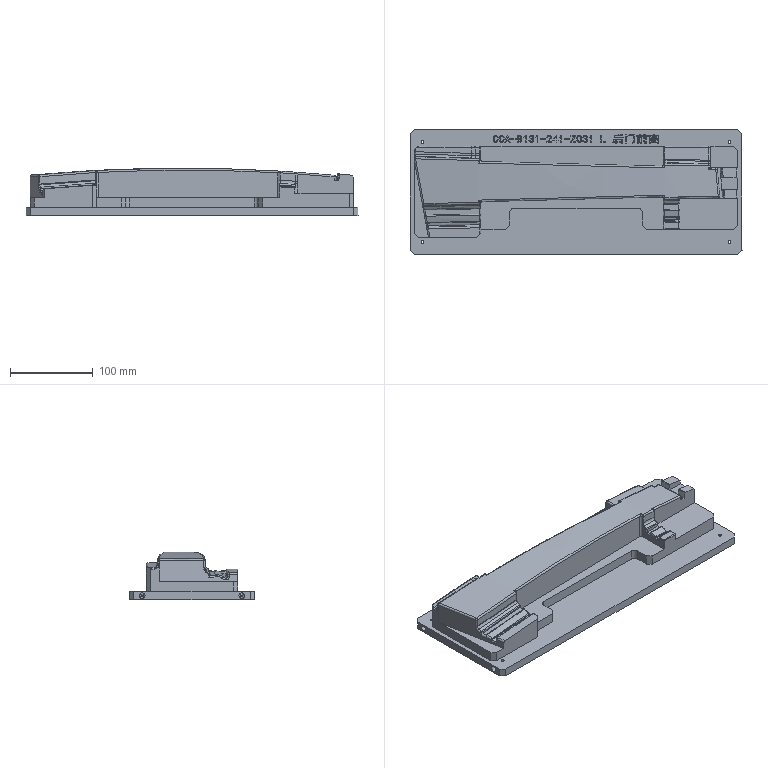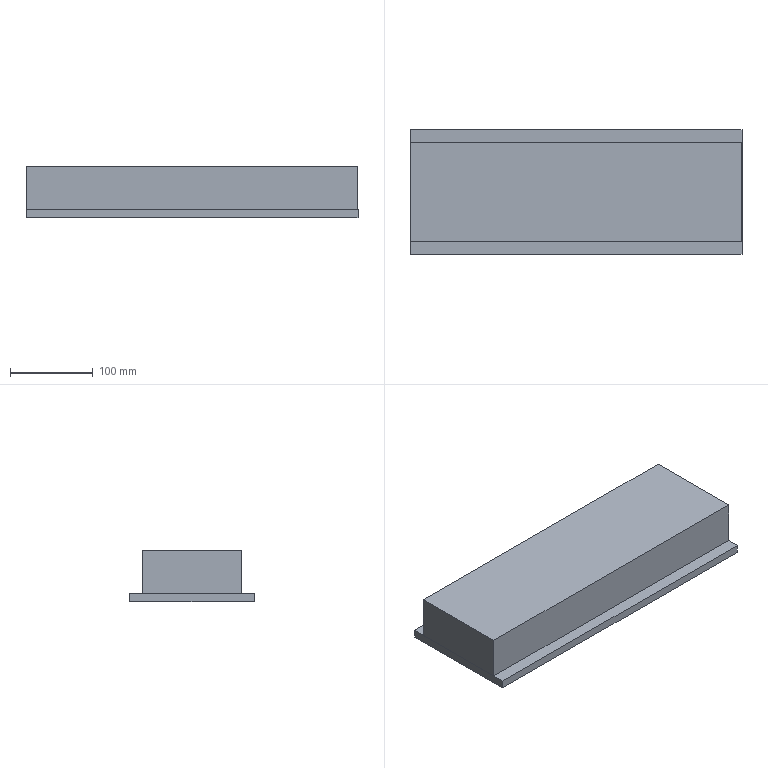CAM job | NX | 3-axis milling, drilling | part box 400 x 150 x 57.494 mm | stock box 400 x 150 x 62.495 mm
Tools:
number,name,description,diameter,corner_radius,flute_length,length,flutes
0,Z4,Drilling Tool,4.0,0.0,35.0,50.0,2
0,Z3.3,Drilling Tool,3.3,0.0,35.0,50.0,2
0,Z5,Drilling Tool,5.0,0.0,35.0,50.0,2
0,D0.5,Milling Tool-5 Parameters,0.5,0.0,50.0,75.0,2
0,D10,Milling Tool-5 Parameters,10.0,0.0,50.0,75.0,2
0,D16,Milling Tool-5 Parameters,16.0,0.0,50.0,75.0,2
0,D6,Milling Tool-5 Parameters,6.0,0.0,50.0,75.0,2
0,D4,Milling Tool-5 Parameters,4.0,0.0,50.0,75.0,2
Operations:
program,operation,operation_type,tool,method,geometry_group,spindle_rpm,surface_speed,feed_per_tooth,feed_cut,feed_plunge,cut_length_mm,path_length_mm,cut_time_min,machine_time_min
BASE_PLATE,A1,Operation,Z4,METHOD,WORKPIECE,1600.0,20.0,0.0469,150.0,0.0,54.0,938.558,0.36,0.4485
BASE_PLATE,A2,Operation,Z5,METHOD,WORKPIECE,1000.0,12.0,0.06,120.0,0.0,104.0,776.099,0.8667,0.9339
BASE_PLATE,A3,Operation,Z3.3,METHOD,WORKPIECE,1200.0,12.0,0.0417,100.0,0.0,52.0,743.087,0.52,0.5891
BASE_PLATE,A4,FaceMilling,D0.5,METHOD,WORKPIECE,0.0,0.0,0.0,250.0,100.0,5923.262,6822.591,23.693,23.783
BASE_PLATE,A5,PlanarMilling,D10,METHOD,WORKPIECE,3500.0,109.0,0.2857,2000.0,100.0,24912.39,25058.897,12.456,12.471
CURVED_SURFACE,B1,CavityMilling,D16,METHOD,WORKPIECE_1,2500.0,125.0,0.6,3000.0,100.0,237367.727,239787.549,79.123,79.365
CURVED_SURFACE,B2,CavityMilling,D6,METHOD,WORKPIECE_1,3500.0,65.0,0.2857,2000.0,100.0,13710.898,22623.992,6.855,7.747
CURVED_SURFACE,B3,FaceMilling,D10,METHOD,WORKPIECE_1,3500.0,109.0,0.1429,1000.0,100.0,785.943,875.943,0.7859,0.7949
CURVED_SURFACE,B4,FaceMilling,D10,METHOD,WORKPIECE_1,3500.0,109.0,0.1429,1000.0,100.0,576.906,656.906,0.5769,0.5849
CURVED_SURFACE,B5,FaceMilling,D10,METHOD,WORKPIECE_1,3500.0,109.0,0.1429,1000.0,100.0,178.716,268.716,0.1787,0.1877
CURVED_SURFACE,B6,FaceMilling,D10,METHOD,WORKPIECE_1,3500.0,109.0,0.1429,1000.0,100.0,204.133,273.133,0.2041,0.211
CURVED_SURFACE,B7,FaceMilling,D10,METHOD,WORKPIECE_1,3500.0,109.0,0.1429,1000.0,100.0,889.698,958.698,0.8897,0.8966
CURVED_SURFACE,B8,ZLevelMilling,D4,METHOD,WORKPIECE_1,4000.0,125.0,0.225,1800.0,100.0,39768.665,43208.717,22.094,22.438